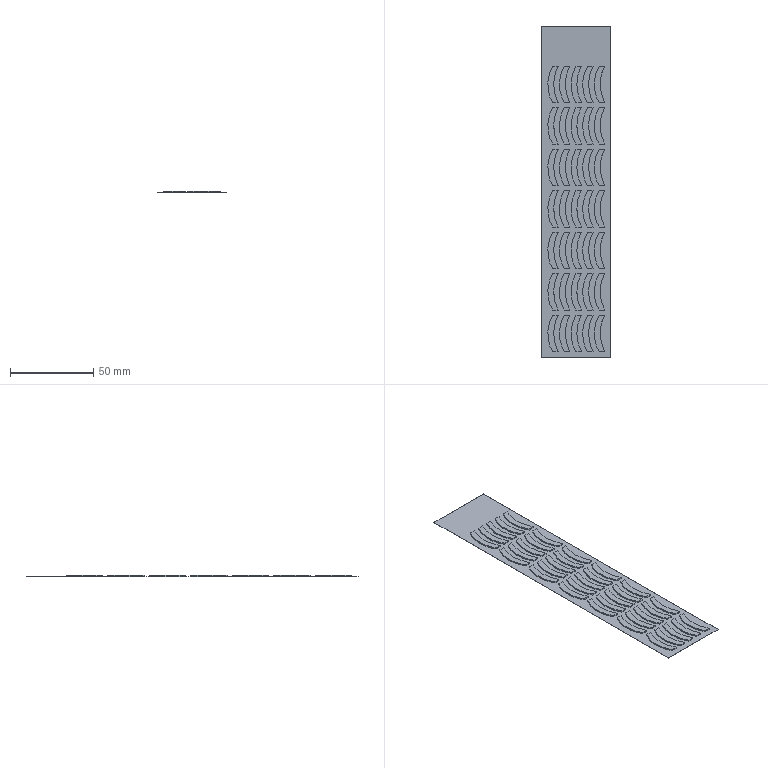Part | STEP file | 10000020486swp000-1 | 1 solid | 181 faces | box 42 x 200 x 0.9 mm | volume 2989 mm3 | plane 111 | spline 70